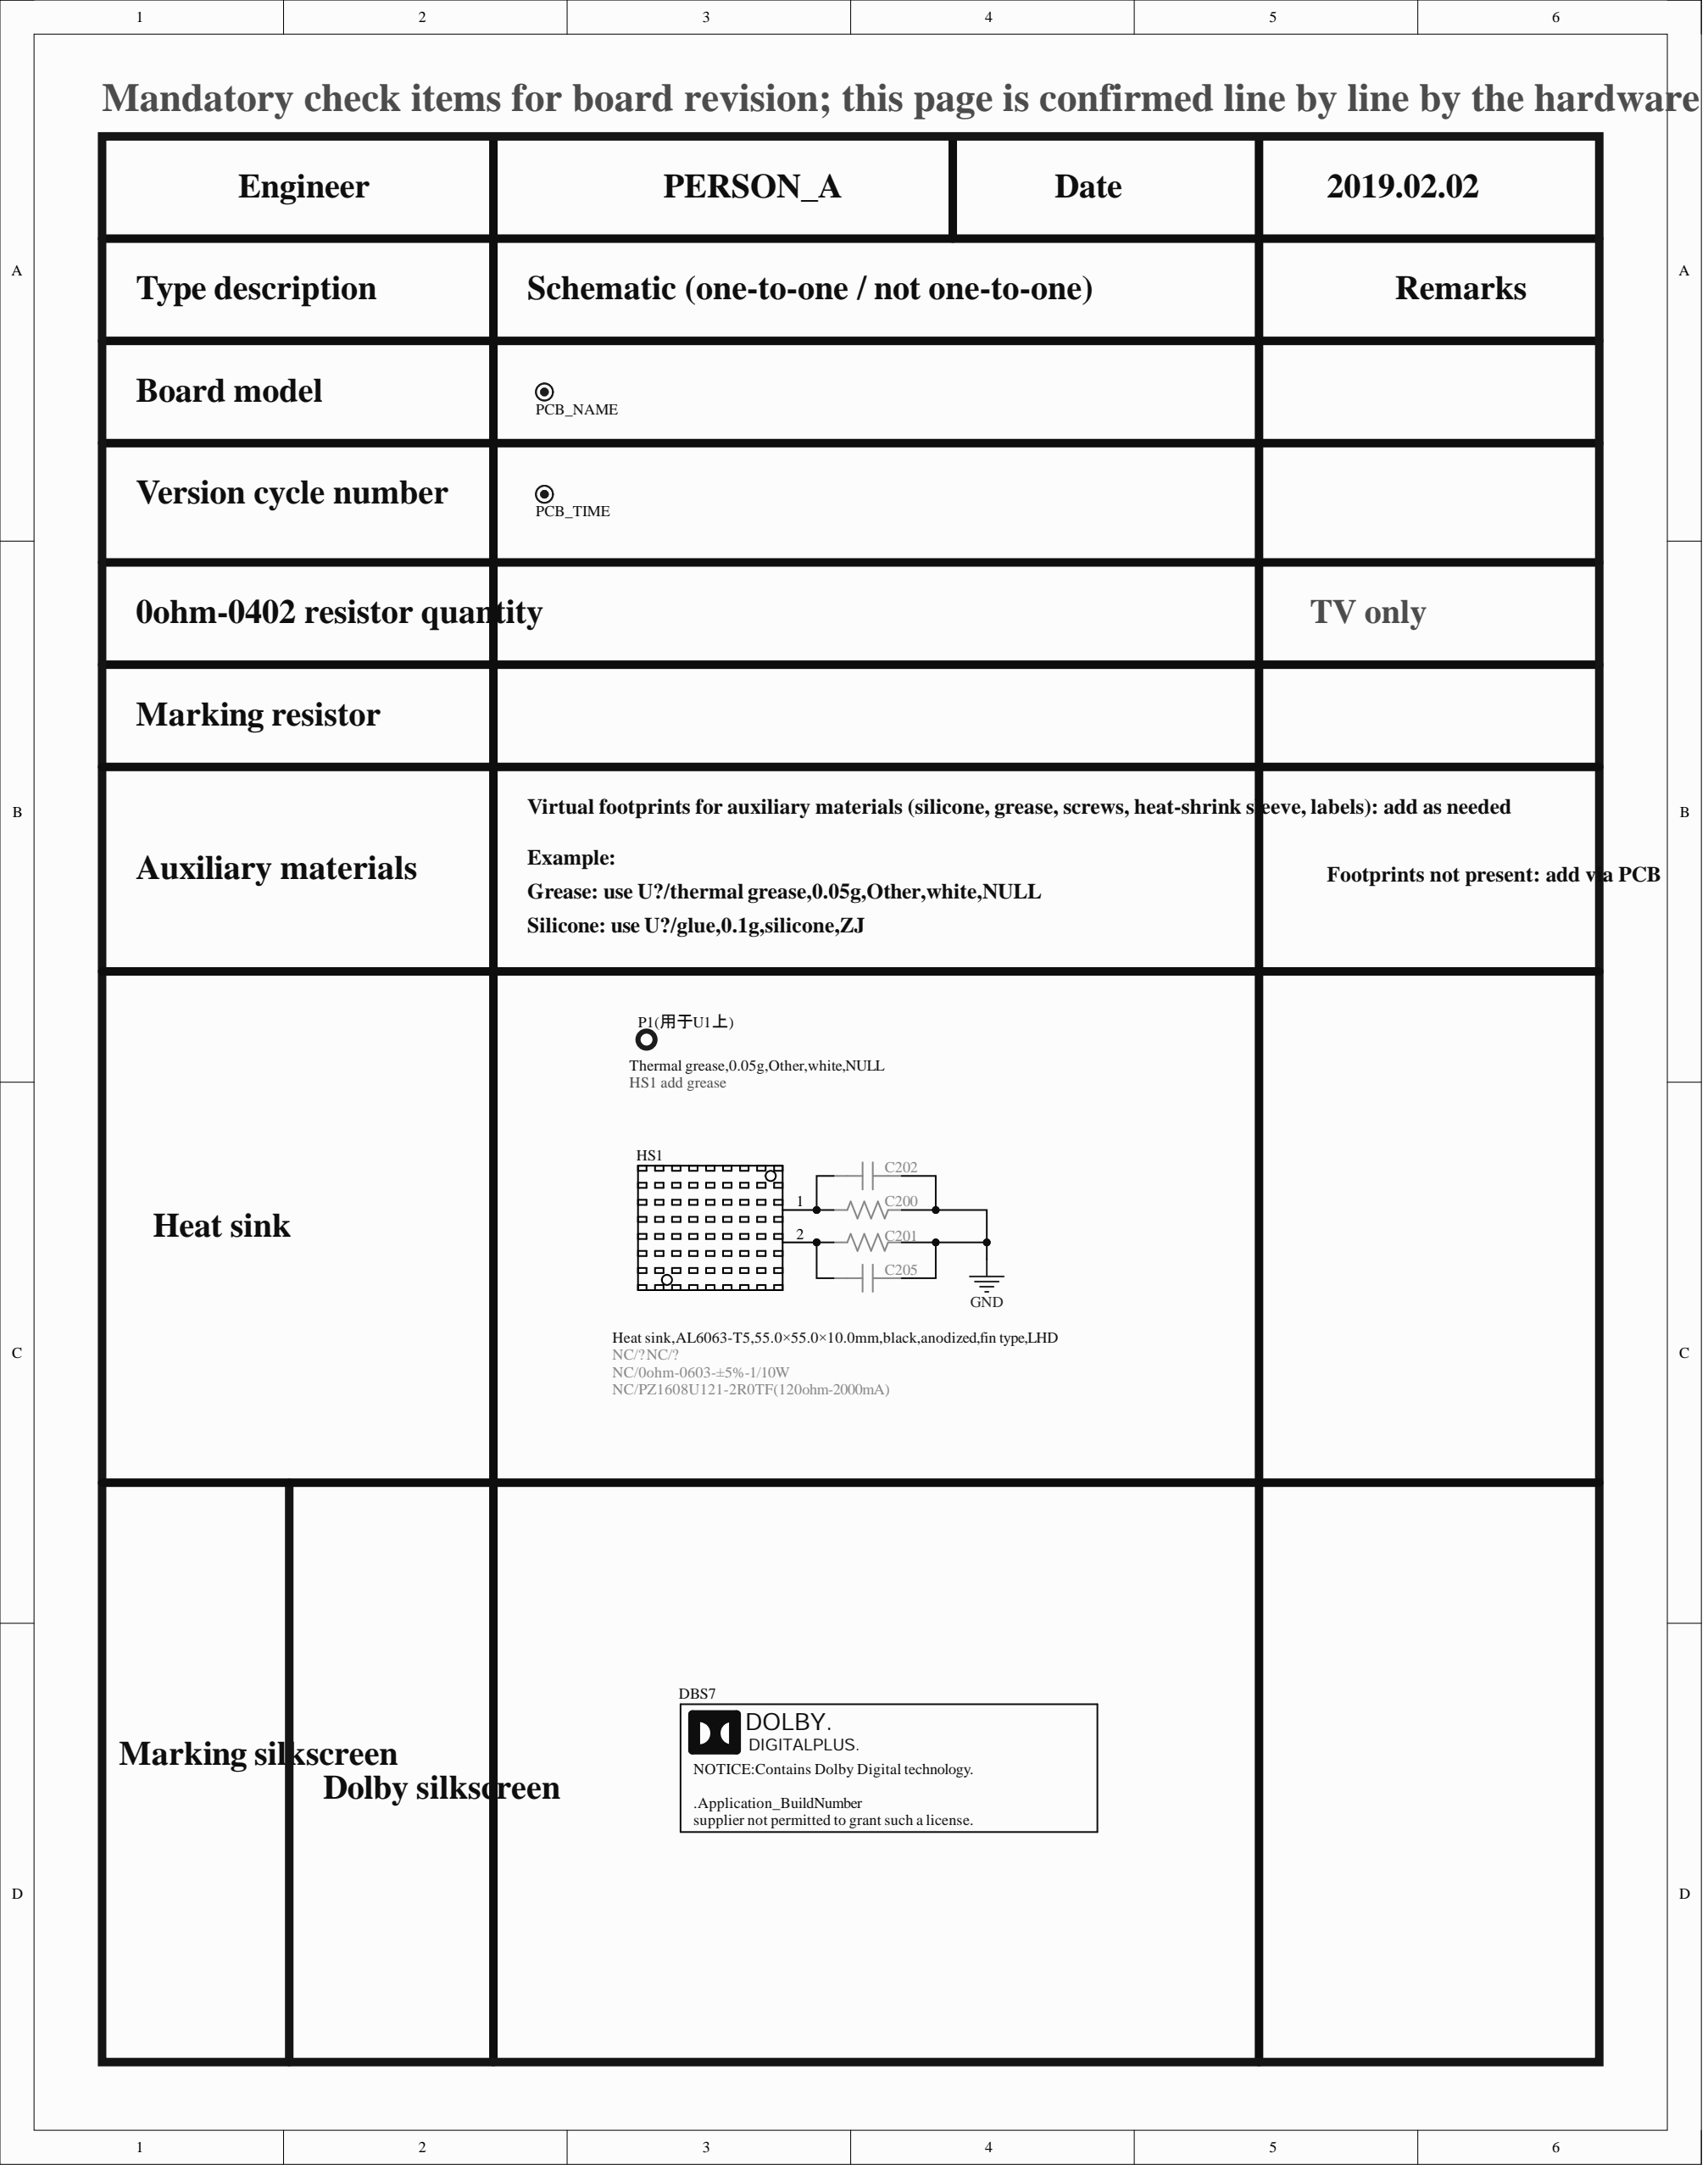Circuit board | Altium Designer | 1029 parts | 642 nets | one sheet of the schematic
Parts on this sheet (reference | value | footprint):
C200 | NC/0ohm-0603-±5%-1/10W | R0603
C201 | NC/PZ1608U121-2R0TF(120ohm-2000mA) | R0603
C202 | NC/? | C0402
C205 | NC/? | C0402
DBS7 | DOLBY PLUS | DOLBY PLUS-SILK
HS1 | Heat sink,AL6063-T5,55.0×55.0×10.0mm,black,anodized,fin type,LHD | HS(55*55*10)
Nets of these parts (net: part-pin ...):
NetC201_2: C201-2 C205-2 HS1-2
NetC200_1: C200-1 C202-2 HS1-1
GND: C200-2 C201-1 C202-1 C205-1